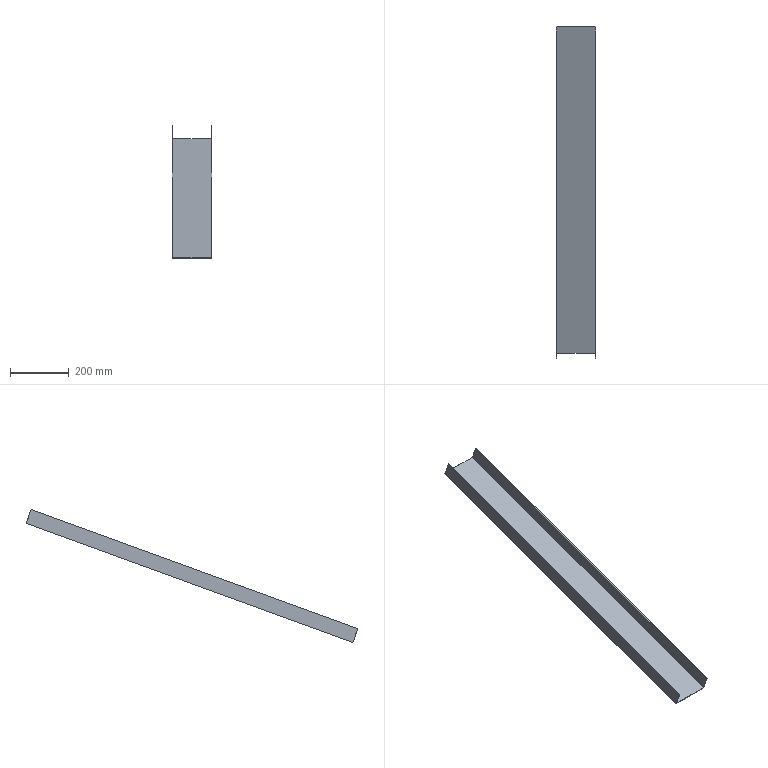Part | NX | features solid 2 | 1 solid | 10 faces | box 133.224 x 1128 x 451.241 mm | volume 541870 mm3 | plane 10
STEP:
#1=CARTESIAN_POINT('',(818.,67.899,-110.15));
#2=VERTEX_POINT('',#1);
#3=CARTESIAN_POINT('',(820.,67.899,-110.15));
#4=VERTEX_POINT('',#3);
#5=CARTESIAN_POINT('',(520.,67.899,-110.15));
#6=DIRECTION('',(1.,0.,0.));
#7=VECTOR('',#6,1000.);
#8=LINE('',#5,#7);
#9=EDGE_CURVE('',#2,#4,#8,.T.);
#10=ORIENTED_EDGE('',*,*,#9,.F.);
#11=CARTESIAN_POINT('',(818.,-1042.785,-514.406));
#12=VERTEX_POINT('',#11);
#13=CARTESIAN_POINT('',(818.,133.237,-86.369));
#14=DIRECTION('',(0.,-0.9397,-0.342));
#15=VECTOR('',#14,1000.);
#16=LINE('',#13,#15);
#17=EDGE_CURVE('',#2,#12,#16,.T.);
#18=ORIENTED_EDGE('',*,*,#17,.T.);
#19=CARTESIAN_POINT('',(820.,-1042.785,-514.406));
#20=VERTEX_POINT('',#19);
#21=CARTESIAN_POINT('',(520.,-1042.785,-514.406));
#22=DIRECTION('',(-1.,0.,0.));
#23=VECTOR('',#22,1000.);
#24=LINE('',#21,#23);
#25=EDGE_CURVE('',#20,#12,#24,.T.);
#26=ORIENTED_EDGE('',*,*,#25,.F.);
#27=CARTESIAN_POINT('',(820.,133.237,-86.369));
#28=DIRECTION('',(0.,-0.9397,-0.342));
#29=VECTOR('',#28,1000.);
#30=LINE('',#27,#29);
#31=EDGE_CURVE('',#4,#20,#30,.T.);
#32=ORIENTED_EDGE('',*,*,#31,.F.);
#33=EDGE_LOOP('',(#10,#18,#26,#32));
#34=FACE_BOUND('',#33,.T.);
#35=CARTESIAN_POINT('',(520.,-547.281,-334.057));
#36=DIRECTION('',(0.,0.342,-0.9397));
#37=DIRECTION('',(-1.,0.,0.));
#38=AXIS2_PLACEMENT_3D('',#35,#36,#37);
#39=PLANE('',#38);
#40=ADVANCED_FACE('',(#34),#39,.F.);
#41=CARTESIAN_POINT('',(686.776,-1042.785,-514.406));
#42=VERTEX_POINT('',#41);
#43=CARTESIAN_POINT('',(686.776,67.899,-110.15));
#44=VERTEX_POINT('',#43);
#45=CARTESIAN_POINT('',(686.776,-130.858,-182.492));
#46=DIRECTION('',(0.,0.9397,0.342));
#47=VECTOR('',#46,1000.);
#48=LINE('',#45,#47);
#49=EDGE_CURVE('',#42,#44,#48,.T.);
#50=ORIENTED_EDGE('',*,*,#49,.T.);
#51=CARTESIAN_POINT('',(686.776,85.,-157.135));
#52=VERTEX_POINT('',#51);
#53=CARTESIAN_POINT('',(686.776,85.,-157.135));
#54=DIRECTION('',(0.,-0.342,0.9397));
#55=VECTOR('',#54,1000.);
#56=LINE('',#53,#55);
#57=EDGE_CURVE('',#52,#44,#56,.T.);
#58=ORIENTED_EDGE('',*,*,#57,.F.);
#59=CARTESIAN_POINT('',(686.776,-1025.684,-561.391));
#60=VERTEX_POINT('',#59);
#61=CARTESIAN_POINT('',(686.776,-113.757,-229.476));
#62=DIRECTION('',(0.,0.9397,0.342));
#63=VECTOR('',#62,1000.);
#64=LINE('',#61,#63);
#65=EDGE_CURVE('',#60,#52,#64,.T.);
#66=ORIENTED_EDGE('',*,*,#65,.F.);
#67=CARTESIAN_POINT('',(686.776,-1101.927,-351.914));
#68=DIRECTION('',(0.,-0.342,0.9397));
#69=VECTOR('',#68,1000.);
#70=LINE('',#67,#69);
#71=EDGE_CURVE('',#60,#42,#70,.T.);
#72=ORIENTED_EDGE('',*,*,#71,.T.);
#73=EDGE_LOOP('',(#50,#58,#66,#72));
#74=FACE_BOUND('',#73,.T.);
#75=CARTESIAN_POINT('',(686.776,-190.,-20.));
#76=DIRECTION('',(1.,0.,0.));
#77=DIRECTION('',(0.,0.,-1.));
#78=AXIS2_PLACEMENT_3D('',#75,#76,#77);
#79=PLANE('',#78);
#80=ADVANCED_FACE('',(#74),#79,.F.);
#81=CARTESIAN_POINT('',(818.,-1026.368,-559.511));
#82=VERTEX_POINT('',#81);
#83=CARTESIAN_POINT('',(688.776,-1026.368,-559.511));
#84=VERTEX_POINT('',#83);
#85=CARTESIAN_POINT('',(520.,-1026.368,-559.511));
#86=DIRECTION('',(-1.,0.,0.));
#87=VECTOR('',#86,1000.);
#88=LINE('',#85,#87);
#89=EDGE_CURVE('',#82,#84,#88,.T.);
#90=ORIENTED_EDGE('',*,*,#89,.T.);
#91=CARTESIAN_POINT('',(688.776,-1042.785,-514.406));
#92=VERTEX_POINT('',#91);
#93=CARTESIAN_POINT('',(688.776,-1101.927,-351.914));
#94=DIRECTION('',(0.,-0.342,0.9397));
#95=VECTOR('',#94,1000.);
#96=LINE('',#93,#95);
#97=EDGE_CURVE('',#84,#92,#96,.T.);
#98=ORIENTED_EDGE('',*,*,#97,.T.);
#99=CARTESIAN_POINT('',(520.,-1042.785,-514.406));
#100=DIRECTION('',(-1.,0.,0.));
#101=VECTOR('',#100,1000.);
#102=LINE('',#99,#101);
#103=EDGE_CURVE('',#92,#42,#102,.T.);
#104=ORIENTED_EDGE('',*,*,#103,.T.);
#105=ORIENTED_EDGE('',*,*,#71,.F.);
#106=CARTESIAN_POINT('',(820.,-1025.684,-561.391));
#107=VERTEX_POINT('',#106);
#108=CARTESIAN_POINT('',(520.,-1025.684,-561.391));
#109=DIRECTION('',(-1.,0.,0.));
#110=VECTOR('',#109,1000.);
#111=LINE('',#108,#110);
#112=EDGE_CURVE('',#107,#60,#111,.T.);
#113=ORIENTED_EDGE('',*,*,#112,.F.);
#114=CARTESIAN_POINT('',(820.,-1025.684,-561.391));
#115=DIRECTION('',(0.,-0.342,0.9397));
#116=VECTOR('',#115,1000.);
#117=LINE('',#114,#116);
#118=EDGE_CURVE('',#107,#20,#117,.T.);
#119=ORIENTED_EDGE('',*,*,#118,.T.);
#120=ORIENTED_EDGE('',*,*,#25,.T.);
#121=CARTESIAN_POINT('',(818.,-1025.684,-561.391));
#122=DIRECTION('',(0.,-0.342,0.9397));
#123=VECTOR('',#122,1000.);
#124=LINE('',#121,#123);
#125=EDGE_CURVE('',#82,#12,#124,.T.);
#126=ORIENTED_EDGE('',*,*,#125,.F.);
#127=EDGE_LOOP('',(#90,#98,#104,#105,#113,#119,#120,#126));
#128=FACE_BOUND('',#127,.T.);
#129=CARTESIAN_POINT('',(520.,-1025.684,-561.391));
#130=DIRECTION('',(0.,0.9397,0.342));
#131=DIRECTION('',(0.,-0.342,0.9397));
#132=AXIS2_PLACEMENT_3D('',#129,#130,#131);
#133=PLANE('',#132);
#134=ADVANCED_FACE('',(#128),#133,.F.);
#135=ORIENTED_EDGE('',*,*,#31,.T.);
#136=ORIENTED_EDGE('',*,*,#118,.F.);
#137=CARTESIAN_POINT('',(820.,85.,-157.135));
#138=VERTEX_POINT('',#137);
#139=CARTESIAN_POINT('',(820.,150.338,-133.354));
#140=DIRECTION('',(0.,-0.9397,-0.342));
#141=VECTOR('',#140,1000.);
#142=LINE('',#139,#141);
#143=EDGE_CURVE('',#138,#107,#142,.T.);
#144=ORIENTED_EDGE('',*,*,#143,.F.);
#145=CARTESIAN_POINT('',(820.,54.662,-73.781));
#146=DIRECTION('',(0.,-0.342,0.9397));
#147=VECTOR('',#146,1000.);
#148=LINE('',#145,#147);
#149=EDGE_CURVE('',#138,#4,#148,.T.);
#150=ORIENTED_EDGE('',*,*,#149,.T.);
#151=EDGE_LOOP('',(#135,#136,#144,#150));
#152=FACE_BOUND('',#151,.T.);
#153=CARTESIAN_POINT('',(820.,120.,-50.));
#154=DIRECTION('',(-1.,0.,0.));
#155=DIRECTION('',(0.,0.,1.));
#156=AXIS2_PLACEMENT_3D('',#153,#154,#155);
#157=PLANE('',#156);
#158=ADVANCED_FACE('',(#152),#157,.F.);
#159=CARTESIAN_POINT('',(688.776,84.316,-155.256));
#160=VERTEX_POINT('',#159);
#161=CARTESIAN_POINT('',(818.,84.316,-155.256));
#162=VERTEX_POINT('',#161);
#163=CARTESIAN_POINT('',(520.,84.316,-155.256));
#164=DIRECTION('',(1.,0.,0.));
#165=VECTOR('',#164,1000.);
#166=LINE('',#163,#165);
#167=EDGE_CURVE('',#160,#162,#166,.T.);
#168=ORIENTED_EDGE('',*,*,#167,.T.);
#169=CARTESIAN_POINT('',(818.,54.662,-73.781));
#170=DIRECTION('',(0.,-0.342,0.9397));
#171=VECTOR('',#170,1000.);
#172=LINE('',#169,#171);
#173=EDGE_CURVE('',#162,#2,#172,.T.);
#174=ORIENTED_EDGE('',*,*,#173,.T.);
#175=ORIENTED_EDGE('',*,*,#9,.T.);
#176=ORIENTED_EDGE('',*,*,#149,.F.);
#177=CARTESIAN_POINT('',(520.,85.,-157.135));
#178=DIRECTION('',(1.,0.,0.));
#179=VECTOR('',#178,1000.);
#180=LINE('',#177,#179);
#181=EDGE_CURVE('',#52,#138,#180,.T.);
#182=ORIENTED_EDGE('',*,*,#181,.F.);
#183=ORIENTED_EDGE('',*,*,#57,.T.);
#184=CARTESIAN_POINT('',(688.776,67.899,-110.15));
#185=VERTEX_POINT('',#184);
#186=CARTESIAN_POINT('',(520.,67.899,-110.15));
#187=DIRECTION('',(1.,0.,0.));
#188=VECTOR('',#187,1000.);
#189=LINE('',#186,#188);
#190=EDGE_CURVE('',#44,#185,#189,.T.);
#191=ORIENTED_EDGE('',*,*,#190,.T.);
#192=CARTESIAN_POINT('',(688.776,85.,-157.135));
#193=DIRECTION('',(0.,-0.342,0.9397));
#194=VECTOR('',#193,1000.);
#195=LINE('',#192,#194);
#196=EDGE_CURVE('',#160,#185,#195,.T.);
#197=ORIENTED_EDGE('',*,*,#196,.F.);
#198=EDGE_LOOP('',(#168,#174,#175,#176,#182,#183,#191,#197));
#199=FACE_BOUND('',#198,.T.);
#200=CARTESIAN_POINT('',(520.,85.,-157.135));
#201=DIRECTION('',(0.,-0.9397,-0.342));
#202=DIRECTION('',(0.,0.342,-0.9397));
#203=AXIS2_PLACEMENT_3D('',#200,#201,#202);
#204=PLANE('',#203);
#205=ADVANCED_FACE('',(#199),#204,.F.);
#206=ORIENTED_EDGE('',*,*,#65,.T.);
#207=ORIENTED_EDGE('',*,*,#181,.T.);
#208=ORIENTED_EDGE('',*,*,#143,.T.);
#209=ORIENTED_EDGE('',*,*,#112,.T.);
#210=EDGE_LOOP('',(#206,#207,#208,#209));
#211=FACE_BOUND('',#210,.T.);
#212=CARTESIAN_POINT('',(520.,-530.18,-381.042));
#213=DIRECTION('',(0.,0.342,-0.9397));
#214=DIRECTION('',(-1.,0.,0.));
#215=AXIS2_PLACEMENT_3D('',#212,#213,#214);
#216=PLANE('',#215);
#217=ADVANCED_FACE('',(#211),#216,.T.);
#218=ORIENTED_EDGE('',*,*,#103,.F.);
#219=CARTESIAN_POINT('',(688.776,-130.858,-182.492));
#220=DIRECTION('',(0.,0.9397,0.342));
#221=VECTOR('',#220,1000.);
#222=LINE('',#219,#221);
#223=EDGE_CURVE('',#92,#185,#222,.T.);
#224=ORIENTED_EDGE('',*,*,#223,.T.);
#225=ORIENTED_EDGE('',*,*,#190,.F.);
#226=ORIENTED_EDGE('',*,*,#49,.F.);
#227=EDGE_LOOP('',(#218,#224,#225,#226));
#228=FACE_BOUND('',#227,.T.);
#229=CARTESIAN_POINT('',(520.,-547.281,-334.057));
#230=DIRECTION('',(0.,0.342,-0.9397));
#231=DIRECTION('',(-1.,0.,0.));
#232=AXIS2_PLACEMENT_3D('',#229,#230,#231);
#233=PLANE('',#232);
#234=ADVANCED_FACE('',(#228),#233,.F.);
#235=ORIENTED_EDGE('',*,*,#223,.F.);
#236=ORIENTED_EDGE('',*,*,#97,.F.);
#237=CARTESIAN_POINT('',(688.776,-114.441,-227.597));
#238=DIRECTION('',(0.,0.9397,0.342));
#239=VECTOR('',#238,1000.);
#240=LINE('',#237,#239);
#241=EDGE_CURVE('',#84,#160,#240,.T.);
#242=ORIENTED_EDGE('',*,*,#241,.T.);
#243=ORIENTED_EDGE('',*,*,#196,.T.);
#244=EDGE_LOOP('',(#235,#236,#242,#243));
#245=FACE_BOUND('',#244,.T.);
#246=CARTESIAN_POINT('',(688.776,-190.,-20.));
#247=DIRECTION('',(1.,0.,0.));
#248=DIRECTION('',(0.,0.,-1.));
#249=AXIS2_PLACEMENT_3D('',#246,#247,#248);
#250=PLANE('',#249);
#251=ADVANCED_FACE('',(#245),#250,.T.);
#252=ORIENTED_EDGE('',*,*,#17,.F.);
#253=ORIENTED_EDGE('',*,*,#173,.F.);
#254=CARTESIAN_POINT('',(818.,149.654,-131.474));
#255=DIRECTION('',(0.,-0.9397,-0.342));
#256=VECTOR('',#255,1000.);
#257=LINE('',#254,#256);
#258=EDGE_CURVE('',#162,#82,#257,.T.);
#259=ORIENTED_EDGE('',*,*,#258,.T.);
#260=ORIENTED_EDGE('',*,*,#125,.T.);
#261=EDGE_LOOP('',(#252,#253,#259,#260));
#262=FACE_BOUND('',#261,.T.);
#263=CARTESIAN_POINT('',(818.,120.,-50.));
#264=DIRECTION('',(-1.,0.,0.));
#265=DIRECTION('',(0.,0.,1.));
#266=AXIS2_PLACEMENT_3D('',#263,#264,#265);
#267=PLANE('',#266);
#268=ADVANCED_FACE('',(#262),#267,.T.);
#269=ORIENTED_EDGE('',*,*,#241,.F.);
#270=ORIENTED_EDGE('',*,*,#89,.F.);
#271=ORIENTED_EDGE('',*,*,#258,.F.);
#272=ORIENTED_EDGE('',*,*,#167,.F.);
#273=EDGE_LOOP('',(#269,#270,#271,#272));
#274=FACE_BOUND('',#273,.T.);
#275=CARTESIAN_POINT('',(520.,-530.864,-379.163));
#276=DIRECTION('',(0.,0.342,-0.9397));
#277=DIRECTION('',(-1.,0.,0.));
#278=AXIS2_PLACEMENT_3D('',#275,#276,#277);
#279=PLANE('',#278);
#280=ADVANCED_FACE('',(#274),#279,.F.);
#281=CLOSED_SHELL('',(#40,#80,#134,#158,#205,#217,#234,#251,#268,#280));
#282=MANIFOLD_SOLID_BREP('',#281);
#283=(LENGTH_UNIT()NAMED_UNIT(*)SI_UNIT(.MILLI.,.METRE.));
#284=UNCERTAINTY_MEASURE_WITH_UNIT(LENGTH_MEASURE(0.00001),#283,'','');
#285=(NAMED_UNIT(*)PLANE_ANGLE_UNIT()SI_UNIT($,.RADIAN.));
#286=(NAMED_UNIT(*)SI_UNIT($,.STERADIAN.)SOLID_ANGLE_UNIT());
#287=(GEOMETRIC_REPRESENTATION_CONTEXT(3)GLOBAL_UNCERTAINTY_ASSIGNED_CONTEXT((#284))GLOBAL_UNIT_ASSIGNED_CONTEXT((#283,#285,#286))REPRESENTATION_CONTEXT('',''));
#288=ADVANCED_BREP_SHAPE_REPRESENTATION('',(#282),#287);